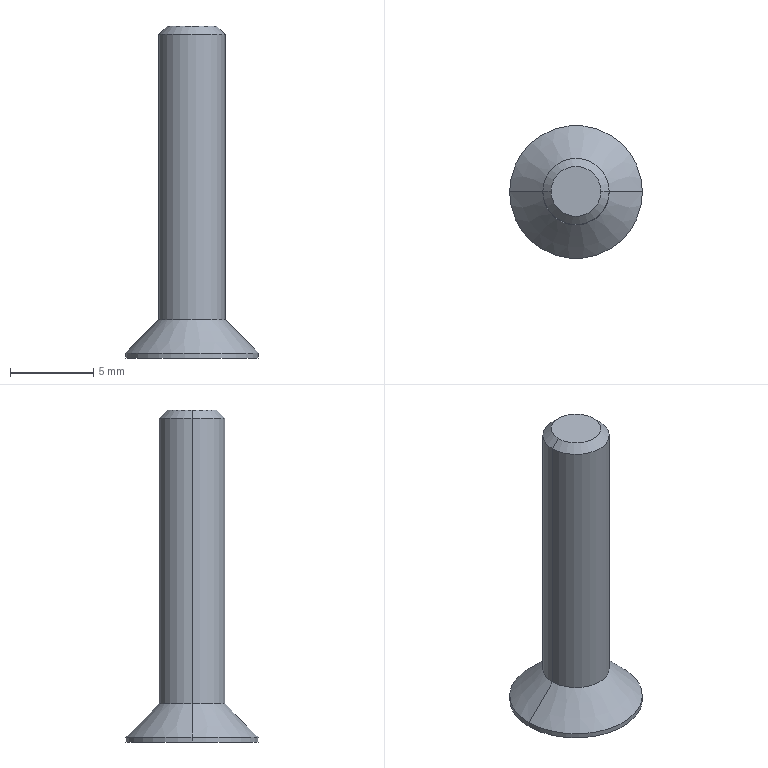Part | SolidWorks | features BaseBody 1 | 1 solid | 24 faces | box 8 x 8 x 20 mm | volume 286.49 mm3 | plane 14 | cone 6 | cylinder 4 | commonest cylinder face diameters 4 x2 8 x2
STEP:
#1=CARTESIAN_POINT('',(-2.,0.,19.5));
#2=VERTEX_POINT('',#1);
#3=CARTESIAN_POINT('',(2.,0.,19.5));
#4=VERTEX_POINT('',#3);
#5=CARTESIAN_POINT('',(0.,0.,19.5));
#6=DIRECTION('',(0.,0.,-1.));
#7=DIRECTION('',(-1.,0.,0.));
#8=AXIS2_PLACEMENT_3D('',#5,#6,#7);
#9=CIRCLE('',#8,2.);
#10=EDGE_CURVE('',#2,#4,#9,.T.);
#11=ORIENTED_EDGE('',*,*,#10,.T.);
#12=CARTESIAN_POINT('',(2.,0.,2.3));
#13=VERTEX_POINT('',#12);
#14=CARTESIAN_POINT('',(2.,0.,20.));
#15=DIRECTION('',(0.,0.,-1.));
#16=VECTOR('',#15,1000.);
#17=LINE('',#14,#16);
#18=EDGE_CURVE('',#4,#13,#17,.T.);
#19=ORIENTED_EDGE('',*,*,#18,.T.);
#20=CARTESIAN_POINT('',(-2.,0.,2.3));
#21=VERTEX_POINT('',#20);
#22=CARTESIAN_POINT('',(0.,0.,2.3));
#23=DIRECTION('',(0.,0.,1.));
#24=DIRECTION('',(-1.,0.,0.));
#25=AXIS2_PLACEMENT_3D('',#22,#23,#24);
#26=CIRCLE('',#25,2.);
#27=EDGE_CURVE('',#13,#21,#26,.T.);
#28=ORIENTED_EDGE('',*,*,#27,.T.);
#29=CARTESIAN_POINT('',(-2.,0.,20.));
#30=DIRECTION('',(0.,0.,-1.));
#31=VECTOR('',#30,1000.);
#32=LINE('',#29,#31);
#33=EDGE_CURVE('',#2,#21,#32,.T.);
#34=ORIENTED_EDGE('',*,*,#33,.F.);
#35=EDGE_LOOP('',(#11,#19,#28,#34));
#36=FACE_OUTER_BOUND('',#35,.T.);
#37=CARTESIAN_POINT('',(0.,0.,20.));
#38=DIRECTION('',(0.,0.,-1.));
#39=DIRECTION('',(-1.,0.,0.));
#40=AXIS2_PLACEMENT_3D('',#37,#38,#39);
#41=CYLINDRICAL_SURFACE('',#40,2.);
#42=ADVANCED_FACE('',(#36),#41,.T.);
#43=ORIENTED_EDGE('',*,*,#27,.F.);
#44=CARTESIAN_POINT('',(4.,0.,0.3));
#45=VERTEX_POINT('',#44);
#46=CARTESIAN_POINT('',(4.,0.,0.3));
#47=DIRECTION('',(0.7071,0.,-0.7071));
#48=VECTOR('',#47,1000.);
#49=LINE('',#46,#48);
#50=EDGE_CURVE('',#13,#45,#49,.T.);
#51=ORIENTED_EDGE('',*,*,#50,.T.);
#52=CARTESIAN_POINT('',(-4.,0.,0.3));
#53=VERTEX_POINT('',#52);
#54=CARTESIAN_POINT('',(0.,0.,0.3));
#55=DIRECTION('',(0.,0.,1.));
#56=DIRECTION('',(-1.,0.,0.));
#57=AXIS2_PLACEMENT_3D('',#54,#55,#56);
#58=CIRCLE('',#57,4.);
#59=EDGE_CURVE('',#45,#53,#58,.T.);
#60=ORIENTED_EDGE('',*,*,#59,.T.);
#61=CARTESIAN_POINT('',(-4.,0.,0.3));
#62=DIRECTION('',(-0.7071,0.,-0.7071));
#63=VECTOR('',#62,1000.);
#64=LINE('',#61,#63);
#65=EDGE_CURVE('',#21,#53,#64,.T.);
#66=ORIENTED_EDGE('',*,*,#65,.F.);
#67=EDGE_LOOP('',(#43,#51,#60,#66));
#68=FACE_OUTER_BOUND('',#67,.T.);
#69=CARTESIAN_POINT('',(0.,0.,0.3));
#70=DIRECTION('',(0.,0.,-1.));
#71=DIRECTION('',(-1.,0.,0.));
#72=AXIS2_PLACEMENT_3D('',#69,#70,#71);
#73=CONICAL_SURFACE('',#72,4.,0.7854);
#74=ADVANCED_FACE('',(#68),#73,.T.);
#75=CARTESIAN_POINT('',(-1.5,0.,20.));
#76=VERTEX_POINT('',#75);
#77=CARTESIAN_POINT('',(1.5,0.,20.));
#78=VERTEX_POINT('',#77);
#79=CARTESIAN_POINT('',(0.,0.,20.));
#80=DIRECTION('',(0.,0.,-1.));
#81=DIRECTION('',(-1.,0.,0.));
#82=AXIS2_PLACEMENT_3D('',#79,#80,#81);
#83=CIRCLE('',#82,1.5);
#84=EDGE_CURVE('',#76,#78,#83,.T.);
#85=ORIENTED_EDGE('',*,*,#84,.T.);
#86=CARTESIAN_POINT('',(2.,0.,19.5));
#87=DIRECTION('',(0.7071,0.,-0.7071));
#88=VECTOR('',#87,1000.);
#89=LINE('',#86,#88);
#90=EDGE_CURVE('',#78,#4,#89,.T.);
#91=ORIENTED_EDGE('',*,*,#90,.T.);
#92=ORIENTED_EDGE('',*,*,#10,.F.);
#93=CARTESIAN_POINT('',(-2.,0.,19.5));
#94=DIRECTION('',(-0.7071,0.,-0.7071));
#95=VECTOR('',#94,1000.);
#96=LINE('',#93,#95);
#97=EDGE_CURVE('',#76,#2,#96,.T.);
#98=ORIENTED_EDGE('',*,*,#97,.F.);
#99=EDGE_LOOP('',(#85,#91,#92,#98));
#100=FACE_OUTER_BOUND('',#99,.T.);
#101=CARTESIAN_POINT('',(0.,0.,19.5));
#102=DIRECTION('',(0.,0.,-1.));
#103=DIRECTION('',(-1.,0.,0.));
#104=AXIS2_PLACEMENT_3D('',#101,#102,#103);
#105=CONICAL_SURFACE('',#104,2.,0.7854);
#106=ADVANCED_FACE('',(#100),#105,.T.);
#107=ORIENTED_EDGE('',*,*,#59,.F.);
#108=CARTESIAN_POINT('',(4.,0.,0.));
#109=VERTEX_POINT('',#108);
#110=CARTESIAN_POINT('',(4.,0.,2.3));
#111=DIRECTION('',(0.,0.,-1.));
#112=VECTOR('',#111,1000.);
#113=LINE('',#110,#112);
#114=EDGE_CURVE('',#45,#109,#113,.T.);
#115=ORIENTED_EDGE('',*,*,#114,.T.);
#116=CARTESIAN_POINT('',(-4.,0.,0.));
#117=VERTEX_POINT('',#116);
#118=CARTESIAN_POINT('',(0.,0.,0.));
#119=DIRECTION('',(0.,0.,1.));
#120=DIRECTION('',(-1.,0.,0.));
#121=AXIS2_PLACEMENT_3D('',#118,#119,#120);
#122=CIRCLE('',#121,4.);
#123=EDGE_CURVE('',#109,#117,#122,.T.);
#124=ORIENTED_EDGE('',*,*,#123,.T.);
#125=CARTESIAN_POINT('',(-4.,0.,2.3));
#126=DIRECTION('',(0.,0.,-1.));
#127=VECTOR('',#126,1000.);
#128=LINE('',#125,#127);
#129=EDGE_CURVE('',#53,#117,#128,.T.);
#130=ORIENTED_EDGE('',*,*,#129,.F.);
#131=EDGE_LOOP('',(#107,#115,#124,#130));
#132=FACE_OUTER_BOUND('',#131,.T.);
#133=CARTESIAN_POINT('',(0.,0.,2.3));
#134=DIRECTION('',(0.,0.,-1.));
#135=DIRECTION('',(-1.,0.,0.));
#136=AXIS2_PLACEMENT_3D('',#133,#134,#135);
#137=CYLINDRICAL_SURFACE('',#136,4.);
#138=ADVANCED_FACE('',(#132),#137,.T.);
#139=CARTESIAN_POINT('',(0.,0.,2.022));
#140=VERTEX_POINT('',#139);
#141=CARTESIAN_POINT('',(-1.25,0.,1.3));
#142=VERTEX_POINT('',#141);
#143=CARTESIAN_POINT('',(-1.25,0.,1.3));
#144=DIRECTION('',(-0.866,0.,-0.5));
#145=VECTOR('',#144,1000.);
#146=LINE('',#143,#145);
#147=EDGE_CURVE('',#140,#142,#146,.T.);
#148=ORIENTED_EDGE('',*,*,#147,.F.);
#149=CARTESIAN_POINT('',(1.25,0.,1.3));
#150=VERTEX_POINT('',#149);
#151=CARTESIAN_POINT('',(1.25,0.,1.3));
#152=DIRECTION('',(0.866,0.,-0.5));
#153=VECTOR('',#152,1000.);
#154=LINE('',#151,#153);
#155=EDGE_CURVE('',#140,#150,#154,.T.);
#156=ORIENTED_EDGE('',*,*,#155,.T.);
#157=CARTESIAN_POINT('',(1.083,-0.625,1.3));
#158=VERTEX_POINT('',#157);
#159=CARTESIAN_POINT('',(0.,0.,1.3));
#160=DIRECTION('',(0.,0.,1.));
#161=DIRECTION('',(-1.,0.,0.));
#162=AXIS2_PLACEMENT_3D('',#159,#160,#161);
#163=CIRCLE('',#162,1.25);
#164=EDGE_CURVE('',#158,#150,#163,.T.);
#165=ORIENTED_EDGE('',*,*,#164,.F.);
#166=CARTESIAN_POINT('',(0.,-1.25,1.3));
#167=VERTEX_POINT('',#166);
#168=CARTESIAN_POINT('',(0.,0.,1.3));
#169=DIRECTION('',(0.,0.,1.));
#170=DIRECTION('',(-1.,0.,0.));
#171=AXIS2_PLACEMENT_3D('',#168,#169,#170);
#172=CIRCLE('',#171,1.25);
#173=EDGE_CURVE('',#167,#158,#172,.T.);
#174=ORIENTED_EDGE('',*,*,#173,.F.);
#175=CARTESIAN_POINT('',(-1.083,-0.625,1.3));
#176=VERTEX_POINT('',#175);
#177=CARTESIAN_POINT('',(0.,0.,1.3));
#178=DIRECTION('',(0.,0.,1.));
#179=DIRECTION('',(-1.,0.,0.));
#180=AXIS2_PLACEMENT_3D('',#177,#178,#179);
#181=CIRCLE('',#180,1.25);
#182=EDGE_CURVE('',#176,#167,#181,.T.);
#183=ORIENTED_EDGE('',*,*,#182,.F.);
#184=CARTESIAN_POINT('',(0.,0.,1.3));
#185=DIRECTION('',(0.,0.,1.));
#186=DIRECTION('',(-1.,0.,0.));
#187=AXIS2_PLACEMENT_3D('',#184,#185,#186);
#188=CIRCLE('',#187,1.25);
#189=EDGE_CURVE('',#142,#176,#188,.T.);
#190=ORIENTED_EDGE('',*,*,#189,.F.);
#191=EDGE_LOOP('',(#148,#156,#165,#174,#183,#190));
#192=FACE_OUTER_BOUND('',#191,.T.);
#193=CARTESIAN_POINT('',(0.,0.,1.3));
#194=DIRECTION('',(0.,0.,-1.));
#195=DIRECTION('',(-1.,0.,0.));
#196=AXIS2_PLACEMENT_3D('',#193,#194,#195);
#197=CONICAL_SURFACE('',#196,1.25,1.047);
#198=ADVANCED_FACE('',(#192),#197,.F.);
#199=ORIENTED_EDGE('',*,*,#18,.F.);
#200=CARTESIAN_POINT('',(0.,0.,19.5));
#201=DIRECTION('',(0.,0.,-1.));
#202=DIRECTION('',(-1.,0.,0.));
#203=AXIS2_PLACEMENT_3D('',#200,#201,#202);
#204=CIRCLE('',#203,2.);
#205=EDGE_CURVE('',#4,#2,#204,.T.);
#206=ORIENTED_EDGE('',*,*,#205,.T.);
#207=ORIENTED_EDGE('',*,*,#33,.T.);
#208=CARTESIAN_POINT('',(0.,0.,2.3));
#209=DIRECTION('',(0.,0.,1.));
#210=DIRECTION('',(-1.,0.,0.));
#211=AXIS2_PLACEMENT_3D('',#208,#209,#210);
#212=CIRCLE('',#211,2.);
#213=EDGE_CURVE('',#21,#13,#212,.T.);
#214=ORIENTED_EDGE('',*,*,#213,.T.);
#215=EDGE_LOOP('',(#199,#206,#207,#214));
#216=FACE_OUTER_BOUND('',#215,.T.);
#217=CARTESIAN_POINT('',(0.,0.,20.));
#218=DIRECTION('',(0.,0.,-1.));
#219=DIRECTION('',(-1.,0.,0.));
#220=AXIS2_PLACEMENT_3D('',#217,#218,#219);
#221=CYLINDRICAL_SURFACE('',#220,2.);
#222=ADVANCED_FACE('',(#216),#221,.T.);
#223=ORIENTED_EDGE('',*,*,#50,.F.);
#224=ORIENTED_EDGE('',*,*,#213,.F.);
#225=ORIENTED_EDGE('',*,*,#65,.T.);
#226=CARTESIAN_POINT('',(0.,0.,0.3));
#227=DIRECTION('',(0.,0.,1.));
#228=DIRECTION('',(-1.,0.,0.));
#229=AXIS2_PLACEMENT_3D('',#226,#227,#228);
#230=CIRCLE('',#229,4.);
#231=EDGE_CURVE('',#53,#45,#230,.T.);
#232=ORIENTED_EDGE('',*,*,#231,.T.);
#233=EDGE_LOOP('',(#223,#224,#225,#232));
#234=FACE_OUTER_BOUND('',#233,.T.);
#235=CARTESIAN_POINT('',(0.,0.,0.3));
#236=DIRECTION('',(0.,0.,-1.));
#237=DIRECTION('',(-1.,0.,0.));
#238=AXIS2_PLACEMENT_3D('',#235,#236,#237);
#239=CONICAL_SURFACE('',#238,4.,0.7854);
#240=ADVANCED_FACE('',(#234),#239,.T.);
#241=ORIENTED_EDGE('',*,*,#90,.F.);
#242=CARTESIAN_POINT('',(0.,0.,20.));
#243=DIRECTION('',(0.,0.,-1.));
#244=DIRECTION('',(-1.,0.,0.));
#245=AXIS2_PLACEMENT_3D('',#242,#243,#244);
#246=CIRCLE('',#245,1.5);
#247=EDGE_CURVE('',#78,#76,#246,.T.);
#248=ORIENTED_EDGE('',*,*,#247,.T.);
#249=ORIENTED_EDGE('',*,*,#97,.T.);
#250=ORIENTED_EDGE('',*,*,#205,.F.);
#251=EDGE_LOOP('',(#241,#248,#249,#250));
#252=FACE_OUTER_BOUND('',#251,.T.);
#253=CARTESIAN_POINT('',(0.,0.,19.5));
#254=DIRECTION('',(0.,0.,-1.));
#255=DIRECTION('',(-1.,0.,0.));
#256=AXIS2_PLACEMENT_3D('',#253,#254,#255);
#257=CONICAL_SURFACE('',#256,2.,0.7854);
#258=ADVANCED_FACE('',(#252),#257,.T.);
#259=ORIENTED_EDGE('',*,*,#114,.F.);
#260=ORIENTED_EDGE('',*,*,#231,.F.);
#261=ORIENTED_EDGE('',*,*,#129,.T.);
#262=CARTESIAN_POINT('',(0.,0.,0.));
#263=DIRECTION('',(0.,0.,1.));
#264=DIRECTION('',(-1.,0.,0.));
#265=AXIS2_PLACEMENT_3D('',#262,#263,#264);
#266=CIRCLE('',#265,4.);
#267=EDGE_CURVE('',#117,#109,#266,.T.);
#268=ORIENTED_EDGE('',*,*,#267,.T.);
#269=EDGE_LOOP('',(#259,#260,#261,#268));
#270=FACE_OUTER_BOUND('',#269,.T.);
#271=CARTESIAN_POINT('',(0.,0.,2.3));
#272=DIRECTION('',(0.,0.,-1.));
#273=DIRECTION('',(-1.,0.,0.));
#274=AXIS2_PLACEMENT_3D('',#271,#272,#273);
#275=CYLINDRICAL_SURFACE('',#274,4.);
#276=ADVANCED_FACE('',(#270),#275,.T.);
#277=ORIENTED_EDGE('',*,*,#84,.F.);
#278=ORIENTED_EDGE('',*,*,#247,.F.);
#279=EDGE_LOOP('',(#277,#278));
#280=FACE_OUTER_BOUND('',#279,.T.);
#281=CARTESIAN_POINT('',(0.,0.,20.));
#282=DIRECTION('',(0.,0.,1.));
#283=DIRECTION('',(1.,0.,0.));
#284=AXIS2_PLACEMENT_3D('',#281,#282,#283);
#285=PLANE('',#284);
#286=ADVANCED_FACE('',(#280),#285,.T.);
#287=ORIENTED_EDGE('',*,*,#267,.F.);
#288=ORIENTED_EDGE('',*,*,#123,.F.);
#289=EDGE_LOOP('',(#287,#288));
#290=FACE_OUTER_BOUND('',#289,.T.);
#291=CARTESIAN_POINT('',(-1.443,0.,0.));
#292=VERTEX_POINT('',#291);
#293=CARTESIAN_POINT('',(-0.7217,1.25,0.));
#294=VERTEX_POINT('',#293);
#295=CARTESIAN_POINT('',(-1.443,0.,0.));
#296=DIRECTION('',(0.5,0.866,0.));
#297=VECTOR('',#296,1000.);
#298=LINE('',#295,#297);
#299=EDGE_CURVE('',#292,#294,#298,.T.);
#300=ORIENTED_EDGE('',*,*,#299,.F.);
#301=CARTESIAN_POINT('',(-0.7217,-1.25,0.));
#302=VERTEX_POINT('',#301);
#303=CARTESIAN_POINT('',(-0.7217,-1.25,0.));
#304=DIRECTION('',(-0.5,0.866,0.));
#305=VECTOR('',#304,1000.);
#306=LINE('',#303,#305);
#307=EDGE_CURVE('',#302,#292,#306,.T.);
#308=ORIENTED_EDGE('',*,*,#307,.F.);
#309=CARTESIAN_POINT('',(0.7217,-1.25,0.));
#310=VERTEX_POINT('',#309);
#311=CARTESIAN_POINT('',(0.,-1.25,0.));
#312=DIRECTION('',(-1.,0.,0.));
#313=VECTOR('',#312,1000.);
#314=LINE('',#311,#313);
#315=EDGE_CURVE('',#310,#302,#314,.T.);
#316=ORIENTED_EDGE('',*,*,#315,.F.);
#317=CARTESIAN_POINT('',(1.443,0.,0.));
#318=VERTEX_POINT('',#317);
#319=CARTESIAN_POINT('',(1.443,0.,0.));
#320=DIRECTION('',(-0.5,-0.866,0.));
#321=VECTOR('',#320,1000.);
#322=LINE('',#319,#321);
#323=EDGE_CURVE('',#318,#310,#322,.T.);
#324=ORIENTED_EDGE('',*,*,#323,.F.);
#325=CARTESIAN_POINT('',(0.7217,1.25,0.));
#326=VERTEX_POINT('',#325);
#327=CARTESIAN_POINT('',(0.7217,1.25,0.));
#328=DIRECTION('',(0.5,-0.866,0.));
#329=VECTOR('',#328,1000.);
#330=LINE('',#327,#329);
#331=EDGE_CURVE('',#326,#318,#330,.T.);
#332=ORIENTED_EDGE('',*,*,#331,.F.);
#333=CARTESIAN_POINT('',(0.,1.25,0.));
#334=DIRECTION('',(1.,0.,0.));
#335=VECTOR('',#334,1000.);
#336=LINE('',#333,#335);
#337=EDGE_CURVE('',#294,#326,#336,.T.);
#338=ORIENTED_EDGE('',*,*,#337,.F.);
#339=EDGE_LOOP('',(#300,#308,#316,#324,#332,#338));
#340=FACE_BOUND('',#339,.T.);
#341=CARTESIAN_POINT('',(0.,0.,0.));
#342=DIRECTION('',(0.,0.,1.));
#343=DIRECTION('',(1.,0.,0.));
#344=AXIS2_PLACEMENT_3D('',#341,#342,#343);
#345=PLANE('',#344);
#346=ADVANCED_FACE('',(#290,#340),#345,.F.);
#347=CARTESIAN_POINT('',(0.7217,1.25,1.3));
#348=VERTEX_POINT('',#347);
#349=CARTESIAN_POINT('',(0.7217,1.25,1.3));
#350=DIRECTION('',(0.,0.,-1.));
#351=VECTOR('',#350,1000.);
#352=LINE('',#349,#351);
#353=EDGE_CURVE('',#348,#326,#352,.T.);
#354=ORIENTED_EDGE('',*,*,#353,.F.);
#355=CARTESIAN_POINT('',(0.,1.25,1.3));
#356=VERTEX_POINT('',#355);
#357=CARTESIAN_POINT('',(-0.7217,1.25,1.3));
#358=DIRECTION('',(1.,0.,0.));
#359=VECTOR('',#358,1000.);
#360=LINE('',#357,#359);
#361=EDGE_CURVE('',#356,#348,#360,.T.);
#362=ORIENTED_EDGE('',*,*,#361,.F.);
#363=CARTESIAN_POINT('',(-0.7217,1.25,1.3));
#364=VERTEX_POINT('',#363);
#365=CARTESIAN_POINT('',(-0.7217,1.25,1.3));
#366=DIRECTION('',(1.,0.,0.));
#367=VECTOR('',#366,1000.);
#368=LINE('',#365,#367);
#369=EDGE_CURVE('',#364,#356,#368,.T.);
#370=ORIENTED_EDGE('',*,*,#369,.F.);
#371=CARTESIAN_POINT('',(-0.7217,1.25,1.3));
#372=DIRECTION('',(0.,0.,1.));
#373=VECTOR('',#372,1000.);
#374=LINE('',#371,#373);
#375=EDGE_CURVE('',#294,#364,#374,.T.);
#376=ORIENTED_EDGE('',*,*,#375,.F.);
#377=ORIENTED_EDGE('',*,*,#337,.T.);
#378=EDGE_LOOP('',(#354,#362,#370,#376,#377));
#379=FACE_OUTER_BOUND('',#378,.T.);
#380=CARTESIAN_POINT('',(-0.7217,1.25,1.3));
#381=DIRECTION('',(0.,1.,0.));
#382=DIRECTION('',(0.,0.,1.));
#383=AXIS2_PLACEMENT_3D('',#380,#381,#382);
#384=PLANE('',#383);
#385=ADVANCED_FACE('',(#379),#384,.F.);
#386=ORIENTED_EDGE('',*,*,#375,.T.);
#387=CARTESIAN_POINT('',(-1.083,0.625,1.3));
#388=VERTEX_POINT('',#387);
#389=CARTESIAN_POINT('',(-1.443,0.,1.3));
#390=DIRECTION('',(0.5,0.866,0.));
#391=VECTOR('',#390,1000.);
#392=LINE('',#389,#391);
#393=EDGE_CURVE('',#388,#364,#392,.T.);
#394=ORIENTED_EDGE('',*,*,#393,.F.);
#395=CARTESIAN_POINT('',(-1.443,0.,1.3));
#396=VERTEX_POINT('',#395);
#397=CARTESIAN_POINT('',(-1.443,0.,1.3));
#398=DIRECTION('',(0.5,0.866,0.));
#399=VECTOR('',#398,1000.);
#400=LINE('',#397,#399);
#401=EDGE_CURVE('',#396,#388,#400,.T.);
#402=ORIENTED_EDGE('',*,*,#401,.F.);
#403=CARTESIAN_POINT('',(-1.443,0.,1.3));
#404=DIRECTION('',(0.,0.,1.));
#405=VECTOR('',#404,1000.);
#406=LINE('',#403,#405);
#407=EDGE_CURVE('',#292,#396,#406,.T.);
#408=ORIENTED_EDGE('',*,*,#407,.F.);
#409=ORIENTED_EDGE('',*,*,#299,.T.);
#410=EDGE_LOOP('',(#386,#394,#402,#408,#409));
#411=FACE_OUTER_BOUND('',#410,.T.);
#412=CARTESIAN_POINT('',(-1.443,0.,1.3));
#413=DIRECTION('',(-0.866,0.5,0.));
#414=DIRECTION('',(-0.5,-0.866,0.));
#415=AXIS2_PLACEMENT_3D('',#412,#413,#414);
#416=PLANE('',#415);
#417=ADVANCED_FACE('',(#411),#416,.F.);
#418=ORIENTED_EDGE('',*,*,#407,.T.);
#419=CARTESIAN_POINT('',(-0.7217,-1.25,1.3));
#420=DIRECTION('',(-0.5,0.866,0.));
#421=VECTOR('',#420,1000.);
#422=LINE('',#419,#421);
#423=EDGE_CURVE('',#176,#396,#422,.T.);
#424=ORIENTED_EDGE('',*,*,#423,.F.);
#425=CARTESIAN_POINT('',(-0.7217,-1.25,1.3));
#426=VERTEX_POINT('',#425);
#427=CARTESIAN_POINT('',(-0.7217,-1.25,1.3));
#428=DIRECTION('',(-0.5,0.866,0.));
#429=VECTOR('',#428,1000.);
#430=LINE('',#427,#429);
#431=EDGE_CURVE('',#426,#176,#430,.T.);
#432=ORIENTED_EDGE('',*,*,#431,.F.);
#433=CARTESIAN_POINT('',(-0.7217,-1.25,1.3));
#434=DIRECTION('',(0.,0.,1.));
#435=VECTOR('',#434,1000.);
#436=LINE('',#433,#435);
#437=EDGE_CURVE('',#302,#426,#436,.T.);
#438=ORIENTED_EDGE('',*,*,#437,.F.);
#439=ORIENTED_EDGE('',*,*,#307,.T.);
#440=EDGE_LOOP('',(#418,#424,#432,#438,#439));
#441=FACE_OUTER_BOUND('',#440,.T.);
#442=CARTESIAN_POINT('',(-0.7217,-1.25,1.3));
#443=DIRECTION('',(-0.866,-0.5,0.));
#444=DIRECTION('',(0.5,-0.866,0.));
#445=AXIS2_PLACEMENT_3D('',#442,#443,#444);
#446=PLANE('',#445);
#447=ADVANCED_FACE('',(#441),#446,.F.);
#448=ORIENTED_EDGE('',*,*,#437,.T.);
#449=CARTESIAN_POINT('',(0.7217,-1.25,1.3));
#450=DIRECTION('',(-1.,0.,0.));
#451=VECTOR('',#450,1000.);
#452=LINE('',#449,#451);
#453=EDGE_CURVE('',#167,#426,#452,.T.);
#454=ORIENTED_EDGE('',*,*,#453,.F.);
#455=CARTESIAN_POINT('',(0.7217,-1.25,1.3));
#456=VERTEX_POINT('',#455);
#457=CARTESIAN_POINT('',(0.7217,-1.25,1.3));
#458=DIRECTION('',(-1.,0.,0.));
#459=VECTOR('',#458,1000.);
#460=LINE('',#457,#459);
#461=EDGE_CURVE('',#456,#167,#460,.T.);
#462=ORIENTED_EDGE('',*,*,#461,.F.);
#463=CARTESIAN_POINT('',(0.7217,-1.25,1.3));
#464=DIRECTION('',(0.,0.,1.));
#465=VECTOR('',#464,1000.);
#466=LINE('',#463,#465);
#467=EDGE_CURVE('',#310,#456,#466,.T.);
#468=ORIENTED_EDGE('',*,*,#467,.F.);
#469=ORIENTED_EDGE('',*,*,#315,.T.);
#470=EDGE_LOOP('',(#448,#454,#462,#468,#469));
#471=FACE_OUTER_BOUND('',#470,.T.);
#472=CARTESIAN_POINT('',(0.7217,-1.25,1.3));
#473=DIRECTION('',(0.,-1.,0.));
#474=DIRECTION('',(0.,0.,-1.));
#475=AXIS2_PLACEMENT_3D('',#472,#473,#474);
#476=PLANE('',#475);
#477=ADVANCED_FACE('',(#471),#476,.F.);
#478=ORIENTED_EDGE('',*,*,#467,.T.);
#479=CARTESIAN_POINT('',(1.443,0.,1.3));
#480=DIRECTION('',(-0.5,-0.866,0.));
#481=VECTOR('',#480,1000.);
#482=LINE('',#479,#481);
#483=EDGE_CURVE('',#158,#456,#482,.T.);
#484=ORIENTED_EDGE('',*,*,#483,.F.);
#485=CARTESIAN_POINT('',(1.443,0.,1.3));
#486=VERTEX_POINT('',#485);
#487=CARTESIAN_POINT('',(1.443,0.,1.3));
#488=DIRECTION('',(-0.5,-0.866,0.));
#489=VECTOR('',#488,1000.);
#490=LINE('',#487,#489);
#491=EDGE_CURVE('',#486,#158,#490,.T.);
#492=ORIENTED_EDGE('',*,*,#491,.F.);
#493=CARTESIAN_POINT('',(1.443,0.,1.3));
#494=DIRECTION('',(0.,0.,1.));
#495=VECTOR('',#494,1000.);
#496=LINE('',#493,#495);
#497=EDGE_CURVE('',#318,#486,#496,.T.);
#498=ORIENTED_EDGE('',*,*,#497,.F.);
#499=ORIENTED_EDGE('',*,*,#323,.T.);
#500=EDGE_LOOP('',(#478,#484,#492,#498,#499));
#501=FACE_OUTER_BOUND('',#500,.T.);
#502=CARTESIAN_POINT('',(1.443,0.,1.3));
#503=DIRECTION('',(0.866,-0.5,0.));
#504=DIRECTION('',(0.5,0.866,0.));
#505=AXIS2_PLACEMENT_3D('',#502,#503,#504);
#506=PLANE('',#505);
#507=ADVANCED_FACE('',(#501),#506,.F.);
#508=ORIENTED_EDGE('',*,*,#497,.T.);
#509=CARTESIAN_POINT('',(1.083,0.625,1.3));
#510=VERTEX_POINT('',#509);
#511=CARTESIAN_POINT('',(0.7217,1.25,1.3));
#512=DIRECTION('',(0.5,-0.866,0.));
#513=VECTOR('',#512,1000.);
#514=LINE('',#511,#513);
#515=EDGE_CURVE('',#510,#486,#514,.T.);
#516=ORIENTED_EDGE('',*,*,#515,.F.);
#517=CARTESIAN_POINT('',(0.7217,1.25,1.3));
#518=DIRECTION('',(0.5,-0.866,0.));
#519=VECTOR('',#518,1000.);
#520=LINE('',#517,#519);
#521=EDGE_CURVE('',#348,#510,#520,.T.);
#522=ORIENTED_EDGE('',*,*,#521,.F.);
#523=ORIENTED_EDGE('',*,*,#353,.T.);
#524=ORIENTED_EDGE('',*,*,#331,.T.);
#525=EDGE_LOOP('',(#508,#516,#522,#523,#524));
#526=FACE_OUTER_BOUND('',#525,.T.);
#527=CARTESIAN_POINT('',(0.7217,1.25,1.3));
#528=DIRECTION('',(0.866,0.5,0.));
#529=DIRECTION('',(-0.5,0.866,0.));
#530=AXIS2_PLACEMENT_3D('',#527,#528,#529);
#531=PLANE('',#530);
#532=ADVANCED_FACE('',(#526),#531,.F.);
#533=ORIENTED_EDGE('',*,*,#361,.T.);
#534=ORIENTED_EDGE('',*,*,#521,.T.);
#535=CARTESIAN_POINT('',(0.,0.,1.3));
#536=DIRECTION('',(0.,0.,1.));
#537=DIRECTION('',(-1.,0.,0.));
#538=AXIS2_PLACEMENT_3D('',#535,#536,#537);
#539=CIRCLE('',#538,1.25);
#540=EDGE_CURVE('',#510,#356,#539,.T.);
#541=ORIENTED_EDGE('',*,*,#540,.T.);
#542=EDGE_LOOP('',(#533,#534,#541));
#543=FACE_OUTER_BOUND('',#542,.T.);
#544=CARTESIAN_POINT('',(0.,0.,1.3));
#545=DIRECTION('',(0.,0.,-1.));
#546=DIRECTION('',(-1.,0.,0.));
#547=AXIS2_PLACEMENT_3D('',#544,#545,#546);
#548=PLANE('',#547);
#549=ADVANCED_FACE('',(#543),#548,.T.);
#550=ORIENTED_EDGE('',*,*,#393,.T.);
#551=ORIENTED_EDGE('',*,*,#369,.T.);
#552=CARTESIAN_POINT('',(0.,0.,1.3));
#553=DIRECTION('',(0.,0.,1.));
#554=DIRECTION('',(-1.,0.,0.));
#555=AXIS2_PLACEMENT_3D('',#552,#553,#554);
#556=CIRCLE('',#555,1.25);
#557=EDGE_CURVE('',#356,#388,#556,.T.);
#558=ORIENTED_EDGE('',*,*,#557,.T.);
#559=EDGE_LOOP('',(#550,#551,#558));
#560=FACE_OUTER_BOUND('',#559,.T.);
#561=CARTESIAN_POINT('',(0.,0.,1.3));
#562=DIRECTION('',(0.,0.,-1.));
#563=DIRECTION('',(-1.,0.,0.));
#564=AXIS2_PLACEMENT_3D('',#561,#562,#563);
#565=PLANE('',#564);
#566=ADVANCED_FACE('',(#560),#565,.T.);
#567=ORIENTED_EDGE('',*,*,#401,.T.);
#568=CARTESIAN_POINT('',(0.,0.,1.3));
#569=DIRECTION('',(0.,0.,1.));
#570=DIRECTION('',(-1.,0.,0.));
#571=AXIS2_PLACEMENT_3D('',#568,#569,#570);
#572=CIRCLE('',#571,1.25);
#573=EDGE_CURVE('',#388,#142,#572,.T.);
#574=ORIENTED_EDGE('',*,*,#573,.T.);
#575=ORIENTED_EDGE('',*,*,#189,.T.);
#576=ORIENTED_EDGE('',*,*,#423,.T.);
#577=EDGE_LOOP('',(#567,#574,#575,#576));
#578=FACE_OUTER_BOUND('',#577,.T.);
#579=CARTESIAN_POINT('',(0.,0.,1.3));
#580=DIRECTION('',(0.,0.,-1.));
#581=DIRECTION('',(-1.,0.,0.));
#582=AXIS2_PLACEMENT_3D('',#579,#580,#581);
#583=PLANE('',#582);
#584=ADVANCED_FACE('',(#578),#583,.T.);
#585=ORIENTED_EDGE('',*,*,#453,.T.);
#586=ORIENTED_EDGE('',*,*,#431,.T.);
#587=ORIENTED_EDGE('',*,*,#182,.T.);
#588=EDGE_LOOP('',(#585,#586,#587));
#589=FACE_OUTER_BOUND('',#588,.T.);
#590=CARTESIAN_POINT('',(0.,0.,1.3));
#591=DIRECTION('',(0.,0.,-1.));
#592=DIRECTION('',(-1.,0.,0.));
#593=AXIS2_PLACEMENT_3D('',#590,#591,#592);
#594=PLANE('',#593);
#595=ADVANCED_FACE('',(#589),#594,.T.);
#596=ORIENTED_EDGE('',*,*,#483,.T.);
#597=ORIENTED_EDGE('',*,*,#461,.T.);
#598=ORIENTED_EDGE('',*,*,#173,.T.);
#599=EDGE_LOOP('',(#596,#597,#598));
#600=FACE_OUTER_BOUND('',#599,.T.);
#601=CARTESIAN_POINT('',(0.,0.,1.3));
#602=DIRECTION('',(0.,0.,-1.));
#603=DIRECTION('',(-1.,0.,0.));
#604=AXIS2_PLACEMENT_3D('',#601,#602,#603);
#605=PLANE('',#604);
#606=ADVANCED_FACE('',(#600),#605,.T.);
#607=ORIENTED_EDGE('',*,*,#491,.T.);
#608=ORIENTED_EDGE('',*,*,#164,.T.);
#609=CARTESIAN_POINT('',(0.,0.,1.3));
#610=DIRECTION('',(0.,0.,1.));
#611=DIRECTION('',(-1.,0.,0.));
#612=AXIS2_PLACEMENT_3D('',#609,#610,#611);
#613=CIRCLE('',#612,1.25);
#614=EDGE_CURVE('',#150,#510,#613,.T.);
#615=ORIENTED_EDGE('',*,*,#614,.T.);
#616=ORIENTED_EDGE('',*,*,#515,.T.);
#617=EDGE_LOOP('',(#607,#608,#615,#616));
#618=FACE_OUTER_BOUND('',#617,.T.);
#619=CARTESIAN_POINT('',(0.,0.,1.3));
#620=DIRECTION('',(0.,0.,-1.));
#621=DIRECTION('',(-1.,0.,0.));
#622=AXIS2_PLACEMENT_3D('',#619,#620,#621);
#623=PLANE('',#622);
#624=ADVANCED_FACE('',(#618),#623,.T.);
#625=ORIENTED_EDGE('',*,*,#155,.F.);
#626=ORIENTED_EDGE('',*,*,#147,.T.);
#627=ORIENTED_EDGE('',*,*,#573,.F.);
#628=ORIENTED_EDGE('',*,*,#557,.F.);
#629=ORIENTED_EDGE('',*,*,#540,.F.);
#630=ORIENTED_EDGE('',*,*,#614,.F.);
#631=EDGE_LOOP('',(#625,#626,#627,#628,#629,#630));
#632=FACE_OUTER_BOUND('',#631,.T.);
#633=CARTESIAN_POINT('',(0.,0.,1.3));
#634=DIRECTION('',(0.,0.,-1.));
#635=DIRECTION('',(-1.,0.,0.));
#636=AXIS2_PLACEMENT_3D('',#633,#634,#635);
#637=CONICAL_SURFACE('',#636,1.25,1.047);
#638=ADVANCED_FACE('',(#632),#637,.F.);
#639=CLOSED_SHELL('',(#42,#74,#106,#138,#198,#222,#240,#258,#276,#286,#346,#385,#417,#447,#477,#507,#532,#549,#566,#584,#595,#606,#624,#638));
#640=MANIFOLD_SOLID_BREP('',#639);
#641=CARTESIAN_POINT('',(0.,0.,0.));
#642=DIRECTION('',(0.,0.,1.));
#643=DIRECTION('',(1.,0.,0.));
#644=AXIS2_PLACEMENT_3D('',#641,#642,#643);
#645=(LENGTH_UNIT()NAMED_UNIT(*)SI_UNIT(.MILLI.,.METRE.));
#646=UNCERTAINTY_MEASURE_WITH_UNIT(LENGTH_MEASURE(0.00001),#645,'','');
#647=(NAMED_UNIT(*)PLANE_ANGLE_UNIT()SI_UNIT($,.RADIAN.));
#648=(NAMED_UNIT(*)SI_UNIT($,.STERADIAN.)SOLID_ANGLE_UNIT());
#649=(GEOMETRIC_REPRESENTATION_CONTEXT(3)GLOBAL_UNCERTAINTY_ASSIGNED_CONTEXT((#646))GLOBAL_UNIT_ASSIGNED_CONTEXT((#645,#647,#648))REPRESENTATION_CONTEXT('',''));
#650=ADVANCED_BREP_SHAPE_REPRESENTATION('',(#640,#644),#649);